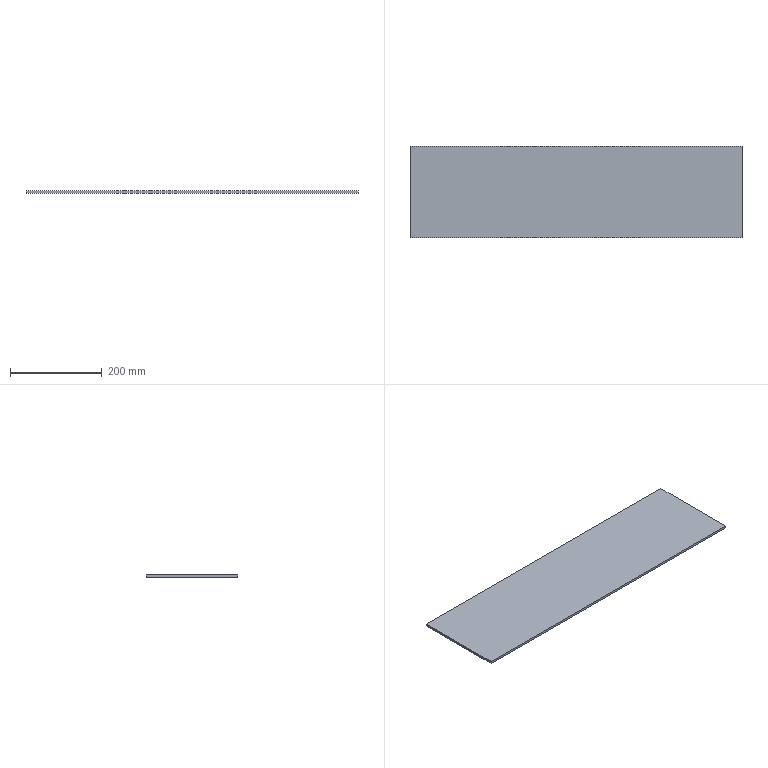Part | NX | features pipe partition 2 | 1 solid | 6 faces | box 723 x 200 x 5 mm | volume 723000 mm3 | plane 6
STEP:
#1=CARTESIAN_POINT('',(-450.,530.,0.));
#2=VERTEX_POINT('',#1);
#3=CARTESIAN_POINT('',(273.,530.,0.));
#4=VERTEX_POINT('',#3);
#5=CARTESIAN_POINT('',(-450.,530.,0.));
#6=DIRECTION('',(1.,0.,0.));
#7=VECTOR('',#6,1000.);
#8=LINE('',#5,#7);
#9=EDGE_CURVE('',#2,#4,#8,.T.);
#10=ORIENTED_EDGE('',*,*,#9,.T.);
#11=CARTESIAN_POINT('',(273.,330.,0.));
#12=VERTEX_POINT('',#11);
#13=CARTESIAN_POINT('',(273.,530.,0.));
#14=DIRECTION('',(0.,1.,0.));
#15=VECTOR('',#14,1000.);
#16=LINE('',#13,#15);
#17=EDGE_CURVE('',#4,#12,#16,.F.);
#18=ORIENTED_EDGE('',*,*,#17,.T.);
#19=CARTESIAN_POINT('',(-450.,330.,0.));
#20=VERTEX_POINT('',#19);
#21=CARTESIAN_POINT('',(-450.,330.,0.));
#22=DIRECTION('',(1.,0.,0.));
#23=VECTOR('',#22,1000.);
#24=LINE('',#21,#23);
#25=EDGE_CURVE('',#12,#20,#24,.F.);
#26=ORIENTED_EDGE('',*,*,#25,.T.);
#27=CARTESIAN_POINT('',(-450.,530.,0.));
#28=DIRECTION('',(0.,1.,0.));
#29=VECTOR('',#28,1000.);
#30=LINE('',#27,#29);
#31=EDGE_CURVE('',#20,#2,#30,.T.);
#32=ORIENTED_EDGE('',*,*,#31,.T.);
#33=EDGE_LOOP('',(#10,#18,#26,#32));
#34=FACE_BOUND('',#33,.T.);
#35=CARTESIAN_POINT('',(-450.,330.,0.));
#36=DIRECTION('',(0.,0.,1.));
#37=DIRECTION('',(1.,0.,0.));
#38=AXIS2_PLACEMENT_3D('',#35,#36,#37);
#39=PLANE('',#38);
#40=ADVANCED_FACE('',(#34),#39,.F.);
#41=CARTESIAN_POINT('',(-450.,330.,5.));
#42=VERTEX_POINT('',#41);
#43=CARTESIAN_POINT('',(-450.,330.,5.));
#44=DIRECTION('',(0.,0.,1.));
#45=VECTOR('',#44,1000.);
#46=LINE('',#43,#45);
#47=EDGE_CURVE('',#20,#42,#46,.T.);
#48=ORIENTED_EDGE('',*,*,#47,.T.);
#49=CARTESIAN_POINT('',(-450.,530.,5.));
#50=VERTEX_POINT('',#49);
#51=CARTESIAN_POINT('',(-450.,330.,5.));
#52=DIRECTION('',(0.,1.,0.));
#53=VECTOR('',#52,1000.);
#54=LINE('',#51,#53);
#55=EDGE_CURVE('',#50,#42,#54,.F.);
#56=ORIENTED_EDGE('',*,*,#55,.F.);
#57=CARTESIAN_POINT('',(-450.,530.,5.));
#58=DIRECTION('',(0.,0.,-1.));
#59=VECTOR('',#58,1000.);
#60=LINE('',#57,#59);
#61=EDGE_CURVE('',#50,#2,#60,.T.);
#62=ORIENTED_EDGE('',*,*,#61,.T.);
#63=ORIENTED_EDGE('',*,*,#31,.F.);
#64=EDGE_LOOP('',(#48,#56,#62,#63));
#65=FACE_BOUND('',#64,.T.);
#66=CARTESIAN_POINT('',(-450.,530.,5.));
#67=DIRECTION('',(1.,0.,0.));
#68=DIRECTION('',(0.,0.,-1.));
#69=AXIS2_PLACEMENT_3D('',#66,#67,#68);
#70=PLANE('',#69);
#71=ADVANCED_FACE('',(#65),#70,.F.);
#72=CARTESIAN_POINT('',(273.,330.,5.));
#73=VERTEX_POINT('',#72);
#74=CARTESIAN_POINT('',(273.,330.,5.));
#75=DIRECTION('',(0.,0.,1.));
#76=VECTOR('',#75,1000.);
#77=LINE('',#74,#76);
#78=EDGE_CURVE('',#12,#73,#77,.T.);
#79=ORIENTED_EDGE('',*,*,#78,.T.);
#80=CARTESIAN_POINT('',(-450.,330.,5.));
#81=DIRECTION('',(1.,0.,0.));
#82=VECTOR('',#81,1000.);
#83=LINE('',#80,#82);
#84=EDGE_CURVE('',#42,#73,#83,.T.);
#85=ORIENTED_EDGE('',*,*,#84,.F.);
#86=ORIENTED_EDGE('',*,*,#47,.F.);
#87=ORIENTED_EDGE('',*,*,#25,.F.);
#88=EDGE_LOOP('',(#79,#85,#86,#87));
#89=FACE_BOUND('',#88,.T.);
#90=CARTESIAN_POINT('',(-450.,330.,5.));
#91=DIRECTION('',(0.,1.,0.));
#92=DIRECTION('',(0.,0.,1.));
#93=AXIS2_PLACEMENT_3D('',#90,#91,#92);
#94=PLANE('',#93);
#95=ADVANCED_FACE('',(#89),#94,.F.);
#96=CARTESIAN_POINT('',(273.,530.,5.));
#97=VERTEX_POINT('',#96);
#98=CARTESIAN_POINT('',(273.,530.,5.));
#99=DIRECTION('',(0.,0.,-1.));
#100=VECTOR('',#99,1000.);
#101=LINE('',#98,#100);
#102=EDGE_CURVE('',#4,#97,#101,.F.);
#103=ORIENTED_EDGE('',*,*,#102,.T.);
#104=CARTESIAN_POINT('',(273.,330.,5.));
#105=DIRECTION('',(0.,1.,0.));
#106=VECTOR('',#105,1000.);
#107=LINE('',#104,#106);
#108=EDGE_CURVE('',#73,#97,#107,.T.);
#109=ORIENTED_EDGE('',*,*,#108,.F.);
#110=ORIENTED_EDGE('',*,*,#78,.F.);
#111=ORIENTED_EDGE('',*,*,#17,.F.);
#112=EDGE_LOOP('',(#103,#109,#110,#111));
#113=FACE_BOUND('',#112,.T.);
#114=CARTESIAN_POINT('',(273.,530.,5.));
#115=DIRECTION('',(-1.,0.,0.));
#116=DIRECTION('',(0.,0.,1.));
#117=AXIS2_PLACEMENT_3D('',#114,#115,#116);
#118=PLANE('',#117);
#119=ADVANCED_FACE('',(#113),#118,.F.);
#120=ORIENTED_EDGE('',*,*,#61,.F.);
#121=CARTESIAN_POINT('',(-450.,530.,5.));
#122=DIRECTION('',(1.,0.,0.));
#123=VECTOR('',#122,1000.);
#124=LINE('',#121,#123);
#125=EDGE_CURVE('',#97,#50,#124,.F.);
#126=ORIENTED_EDGE('',*,*,#125,.F.);
#127=ORIENTED_EDGE('',*,*,#102,.F.);
#128=ORIENTED_EDGE('',*,*,#9,.F.);
#129=EDGE_LOOP('',(#120,#126,#127,#128));
#130=FACE_BOUND('',#129,.T.);
#131=CARTESIAN_POINT('',(-450.,530.,5.));
#132=DIRECTION('',(0.,-1.,0.));
#133=DIRECTION('',(0.,0.,-1.));
#134=AXIS2_PLACEMENT_3D('',#131,#132,#133);
#135=PLANE('',#134);
#136=ADVANCED_FACE('',(#130),#135,.F.);
#137=ORIENTED_EDGE('',*,*,#108,.T.);
#138=ORIENTED_EDGE('',*,*,#125,.T.);
#139=ORIENTED_EDGE('',*,*,#55,.T.);
#140=ORIENTED_EDGE('',*,*,#84,.T.);
#141=EDGE_LOOP('',(#137,#138,#139,#140));
#142=FACE_BOUND('',#141,.T.);
#143=CARTESIAN_POINT('',(-450.,330.,5.));
#144=DIRECTION('',(0.,0.,1.));
#145=DIRECTION('',(1.,0.,0.));
#146=AXIS2_PLACEMENT_3D('',#143,#144,#145);
#147=PLANE('',#146);
#148=ADVANCED_FACE('',(#142),#147,.T.);
#149=CLOSED_SHELL('',(#40,#71,#95,#119,#136,#148));
#150=MANIFOLD_SOLID_BREP('',#149);
#151=(LENGTH_UNIT()NAMED_UNIT(*)SI_UNIT(.MILLI.,.METRE.));
#152=UNCERTAINTY_MEASURE_WITH_UNIT(LENGTH_MEASURE(0.00001),#151,'','');
#153=(NAMED_UNIT(*)PLANE_ANGLE_UNIT()SI_UNIT($,.RADIAN.));
#154=(NAMED_UNIT(*)SI_UNIT($,.STERADIAN.)SOLID_ANGLE_UNIT());
#155=(GEOMETRIC_REPRESENTATION_CONTEXT(3)GLOBAL_UNCERTAINTY_ASSIGNED_CONTEXT((#152))GLOBAL_UNIT_ASSIGNED_CONTEXT((#151,#153,#154))REPRESENTATION_CONTEXT('',''));
#156=ADVANCED_BREP_SHAPE_REPRESENTATION('',(#150),#155);